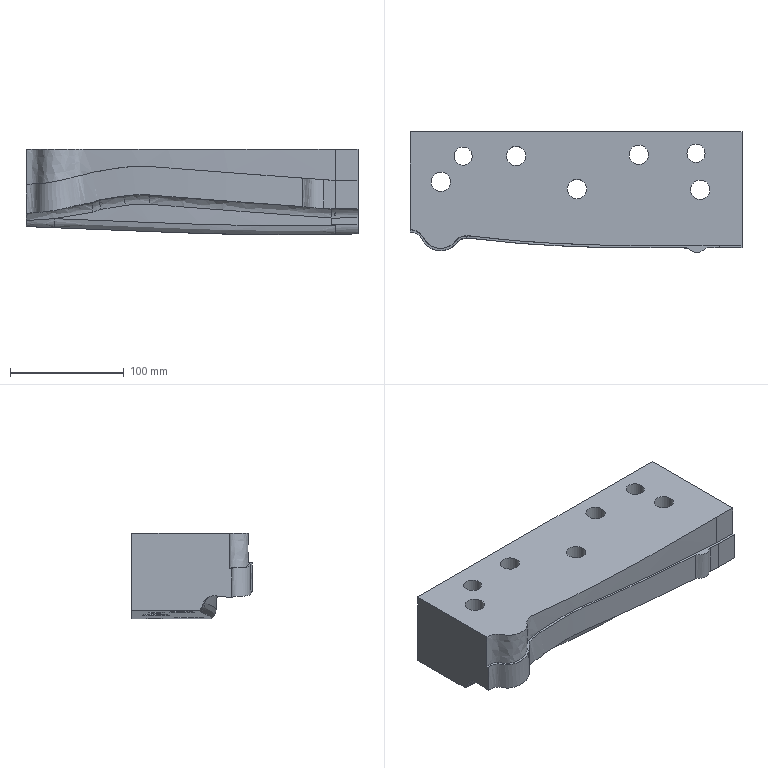Part | NX | features solid 2 | 1 solid | 67 faces | box 291.968 x 106.036 x 75.611 mm | volume 1745971 mm3 | spline 38 | plane 15 | cylinder 14 | commonest cylinder face diameters 17 x7 25 x5 16 x2